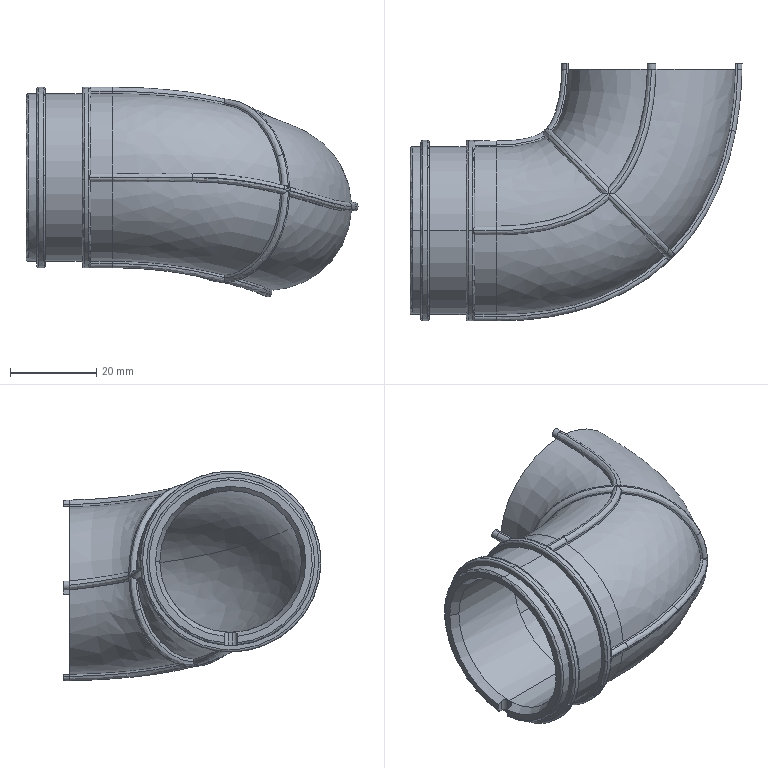Part | STEP file | ZXW722-L-91_1_3_1 | 1 solid | 169 faces | box 76.908 x 59.738 x 48.561 mm | volume 28536 mm3 | spline 78 | plane 41 | cylinder 31 | torus 13 | cone 4 | other 2 | commonest cylinder face diameters 38.835 x8 2 x7 38.82 x4 41.835 x4 1.9 x2 2.001 x2